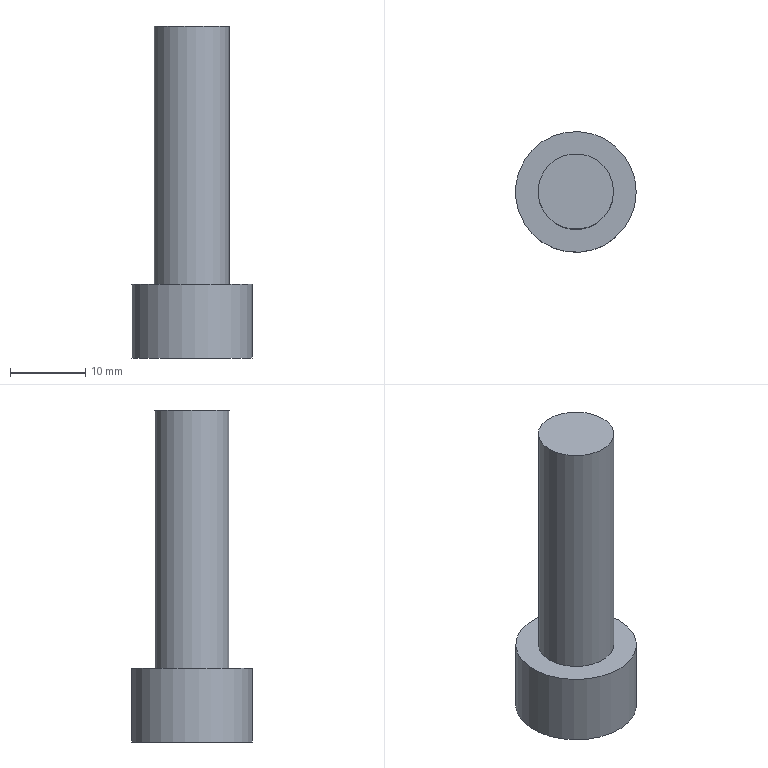Part | NX | features MPPJ 2 | 1 solid | 12 faces | box 16 x 16 x 44 mm | volume 4385 mm3 | plane 10 | cylinder 2 | commonest cylinder face diameters 10 x1 16 x1
STEP:
#1=CARTESIAN_POINT('',(106.,163.,-234.5));
#2=VERTEX_POINT('',#1);
#3=CARTESIAN_POINT('',(98.,163.,-234.5));
#4=DIRECTION('',(0.,0.,1.));
#5=DIRECTION('',(1.,0.,0.));
#6=AXIS2_PLACEMENT_3D('',#3,#4,#5);
#7=CIRCLE('',#6,8.);
#8=EDGE_CURVE('',#2,#2,#7,.T.);
#9=ORIENTED_EDGE('',*,*,#8,.F.);
#10=EDGE_LOOP('',(#9));
#11=FACE_BOUND('',#10,.T.);
#12=CARTESIAN_POINT('',(94.,160.691,-234.5));
#13=VERTEX_POINT('',#12);
#14=CARTESIAN_POINT('',(98.,158.381,-234.5));
#15=VERTEX_POINT('',#14);
#16=CARTESIAN_POINT('',(94.,160.691,-234.5));
#17=DIRECTION('',(0.866,-0.5,0.));
#18=VECTOR('',#17,1000.);
#19=LINE('',#16,#18);
#20=EDGE_CURVE('',#13,#15,#19,.T.);
#21=ORIENTED_EDGE('',*,*,#20,.T.);
#22=CARTESIAN_POINT('',(102.,160.691,-234.5));
#23=VERTEX_POINT('',#22);
#24=CARTESIAN_POINT('',(98.,158.381,-234.5));
#25=DIRECTION('',(0.866,0.5,0.));
#26=VECTOR('',#25,1000.);
#27=LINE('',#24,#26);
#28=EDGE_CURVE('',#15,#23,#27,.T.);
#29=ORIENTED_EDGE('',*,*,#28,.T.);
#30=CARTESIAN_POINT('',(102.,165.309,-234.5));
#31=VERTEX_POINT('',#30);
#32=CARTESIAN_POINT('',(102.,160.691,-234.5));
#33=DIRECTION('',(0.,1.,0.));
#34=VECTOR('',#33,1000.);
#35=LINE('',#32,#34);
#36=EDGE_CURVE('',#23,#31,#35,.T.);
#37=ORIENTED_EDGE('',*,*,#36,.T.);
#38=CARTESIAN_POINT('',(98.,167.619,-234.5));
#39=VERTEX_POINT('',#38);
#40=CARTESIAN_POINT('',(102.,165.309,-234.5));
#41=DIRECTION('',(-0.866,0.5,0.));
#42=VECTOR('',#41,1000.);
#43=LINE('',#40,#42);
#44=EDGE_CURVE('',#31,#39,#43,.T.);
#45=ORIENTED_EDGE('',*,*,#44,.T.);
#46=CARTESIAN_POINT('',(94.,165.309,-234.5));
#47=VERTEX_POINT('',#46);
#48=CARTESIAN_POINT('',(98.,167.619,-234.5));
#49=DIRECTION('',(-0.866,-0.5,0.));
#50=VECTOR('',#49,1000.);
#51=LINE('',#48,#50);
#52=EDGE_CURVE('',#39,#47,#51,.T.);
#53=ORIENTED_EDGE('',*,*,#52,.T.);
#54=CARTESIAN_POINT('',(94.,165.309,-234.5));
#55=DIRECTION('',(0.,-1.,0.));
#56=VECTOR('',#55,1000.);
#57=LINE('',#54,#56);
#58=EDGE_CURVE('',#47,#13,#57,.T.);
#59=ORIENTED_EDGE('',*,*,#58,.T.);
#60=EDGE_LOOP('',(#21,#29,#37,#45,#53,#59));
#61=FACE_BOUND('',#60,.T.);
#62=CARTESIAN_POINT('',(98.,163.,-234.5));
#63=DIRECTION('',(0.,0.,-1.));
#64=DIRECTION('',(-1.,0.,0.));
#65=AXIS2_PLACEMENT_3D('',#62,#63,#64);
#66=PLANE('',#65);
#67=ADVANCED_FACE('',(#11,#61),#66,.T.);
#68=CARTESIAN_POINT('',(103.,163.,-190.5));
#69=VERTEX_POINT('',#68);
#70=CARTESIAN_POINT('',(98.,163.,-190.5));
#71=DIRECTION('',(0.,0.,-1.));
#72=DIRECTION('',(1.,0.,0.));
#73=AXIS2_PLACEMENT_3D('',#70,#71,#72);
#74=CIRCLE('',#73,5.);
#75=EDGE_CURVE('',#69,#69,#74,.T.);
#76=ORIENTED_EDGE('',*,*,#75,.F.);
#77=EDGE_LOOP('',(#76));
#78=FACE_BOUND('',#77,.T.);
#79=CARTESIAN_POINT('',(98.,163.,-190.5));
#80=DIRECTION('',(0.,0.,1.));
#81=DIRECTION('',(1.,0.,0.));
#82=AXIS2_PLACEMENT_3D('',#79,#80,#81);
#83=PLANE('',#82);
#84=ADVANCED_FACE('',(#78),#83,.T.);
#85=CARTESIAN_POINT('',(103.,163.,-224.7));
#86=VERTEX_POINT('',#85);
#87=CARTESIAN_POINT('',(98.,163.,-224.7));
#88=DIRECTION('',(0.,0.,1.));
#89=DIRECTION('',(1.,0.,0.));
#90=AXIS2_PLACEMENT_3D('',#87,#88,#89);
#91=CIRCLE('',#90,5.);
#92=EDGE_CURVE('',#86,#86,#91,.F.);
#93=ORIENTED_EDGE('',*,*,#92,.F.);
#94=EDGE_LOOP('',(#93));
#95=FACE_BOUND('',#94,.T.);
#96=ORIENTED_EDGE('',*,*,#75,.T.);
#97=EDGE_LOOP('',(#96));
#98=FACE_BOUND('',#97,.T.);
#99=CARTESIAN_POINT('',(98.,163.,-234.5));
#100=DIRECTION('',(0.,0.,1.));
#101=DIRECTION('',(1.,0.,0.));
#102=AXIS2_PLACEMENT_3D('',#99,#100,#101);
#103=CYLINDRICAL_SURFACE('',#102,5.);
#104=ADVANCED_FACE('',(#95,#98),#103,.T.);
#105=ORIENTED_EDGE('',*,*,#92,.T.);
#106=EDGE_LOOP('',(#105));
#107=FACE_BOUND('',#106,.T.);
#108=CARTESIAN_POINT('',(106.,163.,-224.7));
#109=VERTEX_POINT('',#108);
#110=CARTESIAN_POINT('',(98.,163.,-224.7));
#111=DIRECTION('',(0.,0.,-1.));
#112=DIRECTION('',(1.,0.,0.));
#113=AXIS2_PLACEMENT_3D('',#110,#111,#112);
#114=CIRCLE('',#113,8.);
#115=EDGE_CURVE('',#109,#109,#114,.T.);
#116=ORIENTED_EDGE('',*,*,#115,.F.);
#117=EDGE_LOOP('',(#116));
#118=FACE_BOUND('',#117,.T.);
#119=CARTESIAN_POINT('',(98.,163.,-224.7));
#120=DIRECTION('',(0.,0.,1.));
#121=DIRECTION('',(1.,0.,0.));
#122=AXIS2_PLACEMENT_3D('',#119,#120,#121);
#123=PLANE('',#122);
#124=ADVANCED_FACE('',(#107,#118),#123,.T.);
#125=ORIENTED_EDGE('',*,*,#115,.T.);
#126=EDGE_LOOP('',(#125));
#127=FACE_BOUND('',#126,.T.);
#128=ORIENTED_EDGE('',*,*,#8,.T.);
#129=EDGE_LOOP('',(#128));
#130=FACE_BOUND('',#129,.T.);
#131=CARTESIAN_POINT('',(98.,163.,-234.5));
#132=DIRECTION('',(0.,0.,1.));
#133=DIRECTION('',(1.,0.,0.));
#134=AXIS2_PLACEMENT_3D('',#131,#132,#133);
#135=CYLINDRICAL_SURFACE('',#134,8.);
#136=ADVANCED_FACE('',(#127,#130),#135,.T.);
#137=CARTESIAN_POINT('',(98.,158.381,-229.6));
#138=VERTEX_POINT('',#137);
#139=CARTESIAN_POINT('',(94.,160.691,-229.6));
#140=VERTEX_POINT('',#139);
#141=CARTESIAN_POINT('',(94.,160.691,-229.6));
#142=DIRECTION('',(0.866,-0.5,0.));
#143=VECTOR('',#142,1000.);
#144=LINE('',#141,#143);
#145=EDGE_CURVE('',#138,#140,#144,.F.);
#146=ORIENTED_EDGE('',*,*,#145,.F.);
#147=CARTESIAN_POINT('',(98.,158.381,-234.5));
#148=DIRECTION('',(0.,0.,1.));
#149=VECTOR('',#148,1000.);
#150=LINE('',#147,#149);
#151=EDGE_CURVE('',#138,#15,#150,.F.);
#152=ORIENTED_EDGE('',*,*,#151,.T.);
#153=ORIENTED_EDGE('',*,*,#20,.F.);
#154=CARTESIAN_POINT('',(94.,160.691,-234.5));
#155=DIRECTION('',(0.,0.,1.));
#156=VECTOR('',#155,1000.);
#157=LINE('',#154,#156);
#158=EDGE_CURVE('',#140,#13,#157,.F.);
#159=ORIENTED_EDGE('',*,*,#158,.F.);
#160=EDGE_LOOP('',(#146,#152,#153,#159));
#161=FACE_BOUND('',#160,.T.);
#162=CARTESIAN_POINT('',(96.,159.536,-232.05));
#163=DIRECTION('',(-0.5,-0.866,0.));
#164=DIRECTION('',(0.866,-0.5,0.));
#165=AXIS2_PLACEMENT_3D('',#162,#163,#164);
#166=PLANE('',#165);
#167=ADVANCED_FACE('',(#161),#166,.F.);
#168=CARTESIAN_POINT('',(94.,165.309,-229.6));
#169=VERTEX_POINT('',#168);
#170=CARTESIAN_POINT('',(94.,165.309,-229.6));
#171=DIRECTION('',(0.,-1.,0.));
#172=VECTOR('',#171,1000.);
#173=LINE('',#170,#172);
#174=EDGE_CURVE('',#140,#169,#173,.F.);
#175=ORIENTED_EDGE('',*,*,#174,.F.);
#176=ORIENTED_EDGE('',*,*,#158,.T.);
#177=ORIENTED_EDGE('',*,*,#58,.F.);
#178=CARTESIAN_POINT('',(94.,165.309,-234.5));
#179=DIRECTION('',(0.,0.,1.));
#180=VECTOR('',#179,1000.);
#181=LINE('',#178,#180);
#182=EDGE_CURVE('',#169,#47,#181,.F.);
#183=ORIENTED_EDGE('',*,*,#182,.F.);
#184=EDGE_LOOP('',(#175,#176,#177,#183));
#185=FACE_BOUND('',#184,.T.);
#186=CARTESIAN_POINT('',(94.,163.,-232.05));
#187=DIRECTION('',(-1.,0.,0.));
#188=DIRECTION('',(0.,0.,1.));
#189=AXIS2_PLACEMENT_3D('',#186,#187,#188);
#190=PLANE('',#189);
#191=ADVANCED_FACE('',(#185),#190,.F.);
#192=CARTESIAN_POINT('',(98.,167.619,-229.6));
#193=VERTEX_POINT('',#192);
#194=CARTESIAN_POINT('',(98.,167.619,-229.6));
#195=DIRECTION('',(-0.866,-0.5,0.));
#196=VECTOR('',#195,1000.);
#197=LINE('',#194,#196);
#198=EDGE_CURVE('',#169,#193,#197,.F.);
#199=ORIENTED_EDGE('',*,*,#198,.F.);
#200=ORIENTED_EDGE('',*,*,#182,.T.);
#201=ORIENTED_EDGE('',*,*,#52,.F.);
#202=CARTESIAN_POINT('',(98.,167.619,-234.5));
#203=DIRECTION('',(0.,0.,1.));
#204=VECTOR('',#203,1000.);
#205=LINE('',#202,#204);
#206=EDGE_CURVE('',#193,#39,#205,.F.);
#207=ORIENTED_EDGE('',*,*,#206,.F.);
#208=EDGE_LOOP('',(#199,#200,#201,#207));
#209=FACE_BOUND('',#208,.T.);
#210=CARTESIAN_POINT('',(96.,166.464,-232.05));
#211=DIRECTION('',(-0.5,0.866,0.));
#212=DIRECTION('',(-0.866,-0.5,0.));
#213=AXIS2_PLACEMENT_3D('',#210,#211,#212);
#214=PLANE('',#213);
#215=ADVANCED_FACE('',(#209),#214,.F.);
#216=CARTESIAN_POINT('',(102.,165.309,-229.6));
#217=VERTEX_POINT('',#216);
#218=CARTESIAN_POINT('',(102.,165.309,-229.6));
#219=DIRECTION('',(-0.866,0.5,0.));
#220=VECTOR('',#219,1000.);
#221=LINE('',#218,#220);
#222=EDGE_CURVE('',#193,#217,#221,.F.);
#223=ORIENTED_EDGE('',*,*,#222,.F.);
#224=ORIENTED_EDGE('',*,*,#206,.T.);
#225=ORIENTED_EDGE('',*,*,#44,.F.);
#226=CARTESIAN_POINT('',(102.,165.309,-234.5));
#227=DIRECTION('',(0.,0.,1.));
#228=VECTOR('',#227,1000.);
#229=LINE('',#226,#228);
#230=EDGE_CURVE('',#217,#31,#229,.F.);
#231=ORIENTED_EDGE('',*,*,#230,.F.);
#232=EDGE_LOOP('',(#223,#224,#225,#231));
#233=FACE_BOUND('',#232,.T.);
#234=CARTESIAN_POINT('',(100.,166.464,-232.05));
#235=DIRECTION('',(0.5,0.866,0.));
#236=DIRECTION('',(-0.866,0.5,0.));
#237=AXIS2_PLACEMENT_3D('',#234,#235,#236);
#238=PLANE('',#237);
#239=ADVANCED_FACE('',(#233),#238,.F.);
#240=CARTESIAN_POINT('',(102.,160.691,-229.6));
#241=VERTEX_POINT('',#240);
#242=CARTESIAN_POINT('',(102.,160.691,-229.6));
#243=DIRECTION('',(0.,1.,0.));
#244=VECTOR('',#243,1000.);
#245=LINE('',#242,#244);
#246=EDGE_CURVE('',#217,#241,#245,.F.);
#247=ORIENTED_EDGE('',*,*,#246,.F.);
#248=ORIENTED_EDGE('',*,*,#230,.T.);
#249=ORIENTED_EDGE('',*,*,#36,.F.);
#250=CARTESIAN_POINT('',(102.,160.691,-234.5));
#251=DIRECTION('',(0.,0.,1.));
#252=VECTOR('',#251,1000.);
#253=LINE('',#250,#252);
#254=EDGE_CURVE('',#241,#23,#253,.F.);
#255=ORIENTED_EDGE('',*,*,#254,.F.);
#256=EDGE_LOOP('',(#247,#248,#249,#255));
#257=FACE_BOUND('',#256,.T.);
#258=CARTESIAN_POINT('',(102.,163.,-232.05));
#259=DIRECTION('',(1.,0.,0.));
#260=DIRECTION('',(0.,0.,-1.));
#261=AXIS2_PLACEMENT_3D('',#258,#259,#260);
#262=PLANE('',#261);
#263=ADVANCED_FACE('',(#257),#262,.F.);
#264=CARTESIAN_POINT('',(98.,158.381,-229.6));
#265=DIRECTION('',(0.866,0.5,0.));
#266=VECTOR('',#265,1000.);
#267=LINE('',#264,#266);
#268=EDGE_CURVE('',#241,#138,#267,.F.);
#269=ORIENTED_EDGE('',*,*,#268,.F.);
#270=ORIENTED_EDGE('',*,*,#254,.T.);
#271=ORIENTED_EDGE('',*,*,#28,.F.);
#272=ORIENTED_EDGE('',*,*,#151,.F.);
#273=EDGE_LOOP('',(#269,#270,#271,#272));
#274=FACE_BOUND('',#273,.T.);
#275=CARTESIAN_POINT('',(100.,159.536,-232.05));
#276=DIRECTION('',(0.5,-0.866,0.));
#277=DIRECTION('',(0.866,0.5,0.));
#278=AXIS2_PLACEMENT_3D('',#275,#276,#277);
#279=PLANE('',#278);
#280=ADVANCED_FACE('',(#274),#279,.F.);
#281=ORIENTED_EDGE('',*,*,#174,.T.);
#282=ORIENTED_EDGE('',*,*,#198,.T.);
#283=ORIENTED_EDGE('',*,*,#222,.T.);
#284=ORIENTED_EDGE('',*,*,#246,.T.);
#285=ORIENTED_EDGE('',*,*,#268,.T.);
#286=ORIENTED_EDGE('',*,*,#145,.T.);
#287=EDGE_LOOP('',(#281,#282,#283,#284,#285,#286));
#288=FACE_BOUND('',#287,.T.);
#289=CARTESIAN_POINT('',(98.,163.,-229.6));
#290=DIRECTION('',(0.,0.,1.));
#291=DIRECTION('',(1.,0.,0.));
#292=AXIS2_PLACEMENT_3D('',#289,#290,#291);
#293=PLANE('',#292);
#294=ADVANCED_FACE('',(#288),#293,.F.);
#295=CLOSED_SHELL('',(#67,#84,#104,#124,#136,#167,#191,#215,#239,#263,#280,#294));
#296=MANIFOLD_SOLID_BREP('',#295);
#297=(LENGTH_UNIT()NAMED_UNIT(*)SI_UNIT(.MILLI.,.METRE.));
#298=UNCERTAINTY_MEASURE_WITH_UNIT(LENGTH_MEASURE(0.00001),#297,'','');
#299=(NAMED_UNIT(*)PLANE_ANGLE_UNIT()SI_UNIT($,.RADIAN.));
#300=(NAMED_UNIT(*)SI_UNIT($,.STERADIAN.)SOLID_ANGLE_UNIT());
#301=(GEOMETRIC_REPRESENTATION_CONTEXT(3)GLOBAL_UNCERTAINTY_ASSIGNED_CONTEXT((#298))GLOBAL_UNIT_ASSIGNED_CONTEXT((#297,#299,#300))REPRESENTATION_CONTEXT('',''));
#302=ADVANCED_BREP_SHAPE_REPRESENTATION('',(#296),#301);